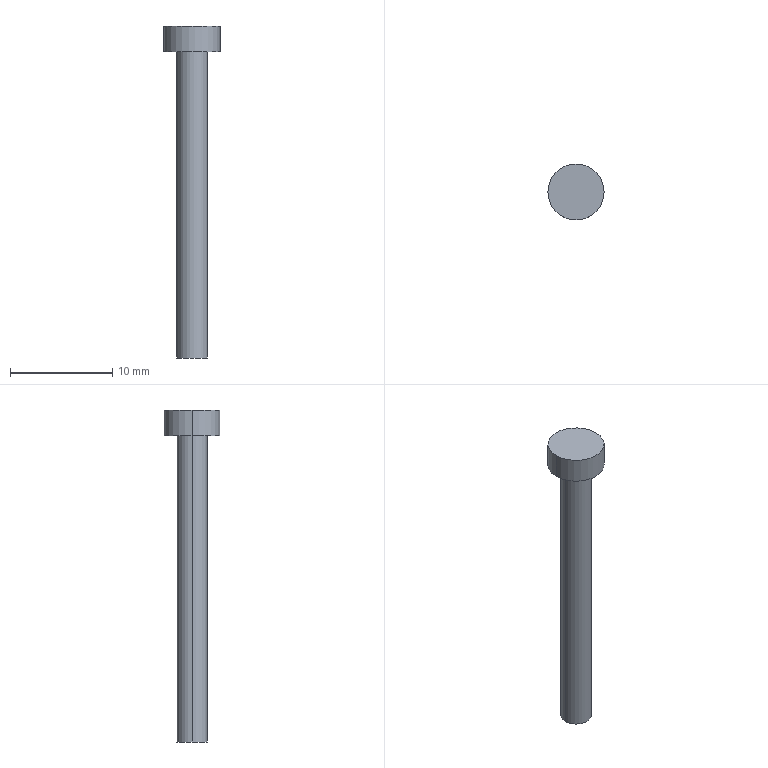Part | SolidWorks | features Extrusion 1, ICE 1 | 1 solid | 7 faces | box 5.5 x 5.5 x 32.5 mm | volume 271.453 mm3 | cylinder 4 | plane 3 | commonest cylinder face diameters 3 x2 5.5 x2
STEP:
#1=CARTESIAN_POINT('',(2.75,0.,2.5));
#2=VERTEX_POINT('',#1);
#3=CARTESIAN_POINT('',(-2.75,0.,2.5));
#4=VERTEX_POINT('',#3);
#5=CARTESIAN_POINT('',(0.,0.,2.5));
#6=DIRECTION('',(0.,0.,1.));
#7=DIRECTION('',(1.,0.,0.));
#8=AXIS2_PLACEMENT_3D('',#5,#6,#7);
#9=CIRCLE('',#8,2.75);
#10=EDGE_CURVE('',#2,#4,#9,.T.);
#11=ORIENTED_EDGE('',*,*,#10,.F.);
#12=CARTESIAN_POINT('',(2.75,0.,0.));
#13=VERTEX_POINT('',#12);
#14=CARTESIAN_POINT('',(2.75,0.,2.5));
#15=DIRECTION('',(0.,0.,-1.));
#16=VECTOR('',#15,1000.);
#17=LINE('',#14,#16);
#18=EDGE_CURVE('',#2,#13,#17,.T.);
#19=ORIENTED_EDGE('',*,*,#18,.T.);
#20=CARTESIAN_POINT('',(-2.75,0.,0.));
#21=VERTEX_POINT('',#20);
#22=CARTESIAN_POINT('',(0.,0.,0.));
#23=DIRECTION('',(0.,0.,1.));
#24=DIRECTION('',(1.,0.,0.));
#25=AXIS2_PLACEMENT_3D('',#22,#23,#24);
#26=CIRCLE('',#25,2.75);
#27=EDGE_CURVE('',#13,#21,#26,.T.);
#28=ORIENTED_EDGE('',*,*,#27,.T.);
#29=CARTESIAN_POINT('',(-2.75,0.,2.5));
#30=DIRECTION('',(0.,0.,-1.));
#31=VECTOR('',#30,1000.);
#32=LINE('',#29,#31);
#33=EDGE_CURVE('',#4,#21,#32,.T.);
#34=ORIENTED_EDGE('',*,*,#33,.F.);
#35=EDGE_LOOP('',(#11,#19,#28,#34));
#36=FACE_OUTER_BOUND('',#35,.T.);
#37=CARTESIAN_POINT('',(0.,0.,2.5));
#38=DIRECTION('',(0.,0.,-1.));
#39=DIRECTION('',(-1.,0.,0.));
#40=AXIS2_PLACEMENT_3D('',#37,#38,#39);
#41=CYLINDRICAL_SURFACE('',#40,2.75);
#42=ADVANCED_FACE('',(#36),#41,.T.);
#43=CARTESIAN_POINT('',(1.5,0.,-30.));
#44=VERTEX_POINT('',#43);
#45=CARTESIAN_POINT('',(-1.5,0.,-30.));
#46=VERTEX_POINT('',#45);
#47=CARTESIAN_POINT('',(0.,0.,-30.));
#48=DIRECTION('',(0.,0.,1.));
#49=DIRECTION('',(1.,0.,0.));
#50=AXIS2_PLACEMENT_3D('',#47,#48,#49);
#51=CIRCLE('',#50,1.5);
#52=EDGE_CURVE('',#44,#46,#51,.T.);
#53=ORIENTED_EDGE('',*,*,#52,.T.);
#54=CARTESIAN_POINT('',(-1.5,0.,0.));
#55=VERTEX_POINT('',#54);
#56=CARTESIAN_POINT('',(-1.5,0.,-30.));
#57=DIRECTION('',(0.,0.,1.));
#58=VECTOR('',#57,1000.);
#59=LINE('',#56,#58);
#60=EDGE_CURVE('',#46,#55,#59,.T.);
#61=ORIENTED_EDGE('',*,*,#60,.T.);
#62=CARTESIAN_POINT('',(1.5,0.,0.));
#63=VERTEX_POINT('',#62);
#64=CARTESIAN_POINT('',(0.,0.,0.));
#65=DIRECTION('',(0.,0.,1.));
#66=DIRECTION('',(1.,0.,0.));
#67=AXIS2_PLACEMENT_3D('',#64,#65,#66);
#68=CIRCLE('',#67,1.5);
#69=EDGE_CURVE('',#63,#55,#68,.T.);
#70=ORIENTED_EDGE('',*,*,#69,.F.);
#71=CARTESIAN_POINT('',(1.5,0.,-30.));
#72=DIRECTION('',(0.,0.,1.));
#73=VECTOR('',#72,1000.);
#74=LINE('',#71,#73);
#75=EDGE_CURVE('',#44,#63,#74,.T.);
#76=ORIENTED_EDGE('',*,*,#75,.F.);
#77=EDGE_LOOP('',(#53,#61,#70,#76));
#78=FACE_OUTER_BOUND('',#77,.T.);
#79=CARTESIAN_POINT('',(0.,0.,-30.));
#80=DIRECTION('',(0.,0.,1.));
#81=DIRECTION('',(1.,0.,0.));
#82=AXIS2_PLACEMENT_3D('',#79,#80,#81);
#83=CYLINDRICAL_SURFACE('',#82,1.5);
#84=ADVANCED_FACE('',(#78),#83,.T.);
#85=ORIENTED_EDGE('',*,*,#60,.F.);
#86=CARTESIAN_POINT('',(0.,0.,-30.));
#87=DIRECTION('',(0.,0.,1.));
#88=DIRECTION('',(1.,0.,0.));
#89=AXIS2_PLACEMENT_3D('',#86,#87,#88);
#90=CIRCLE('',#89,1.5);
#91=EDGE_CURVE('',#46,#44,#90,.T.);
#92=ORIENTED_EDGE('',*,*,#91,.T.);
#93=ORIENTED_EDGE('',*,*,#75,.T.);
#94=CARTESIAN_POINT('',(0.,0.,0.));
#95=DIRECTION('',(0.,0.,1.));
#96=DIRECTION('',(1.,0.,0.));
#97=AXIS2_PLACEMENT_3D('',#94,#95,#96);
#98=CIRCLE('',#97,1.5);
#99=EDGE_CURVE('',#55,#63,#98,.T.);
#100=ORIENTED_EDGE('',*,*,#99,.F.);
#101=EDGE_LOOP('',(#85,#92,#93,#100));
#102=FACE_OUTER_BOUND('',#101,.T.);
#103=CARTESIAN_POINT('',(0.,0.,-30.));
#104=DIRECTION('',(0.,0.,1.));
#105=DIRECTION('',(1.,0.,0.));
#106=AXIS2_PLACEMENT_3D('',#103,#104,#105);
#107=CYLINDRICAL_SURFACE('',#106,1.5);
#108=ADVANCED_FACE('',(#102),#107,.T.);
#109=ORIENTED_EDGE('',*,*,#52,.F.);
#110=ORIENTED_EDGE('',*,*,#91,.F.);
#111=EDGE_LOOP('',(#109,#110));
#112=FACE_OUTER_BOUND('',#111,.T.);
#113=CARTESIAN_POINT('',(0.,0.,-30.));
#114=DIRECTION('',(0.,0.,1.));
#115=DIRECTION('',(1.,0.,0.));
#116=AXIS2_PLACEMENT_3D('',#113,#114,#115);
#117=PLANE('',#116);
#118=ADVANCED_FACE('',(#112),#117,.F.);
#119=ORIENTED_EDGE('',*,*,#18,.F.);
#120=CARTESIAN_POINT('',(0.,0.,2.5));
#121=DIRECTION('',(0.,0.,1.));
#122=DIRECTION('',(1.,0.,0.));
#123=AXIS2_PLACEMENT_3D('',#120,#121,#122);
#124=CIRCLE('',#123,2.75);
#125=EDGE_CURVE('',#4,#2,#124,.T.);
#126=ORIENTED_EDGE('',*,*,#125,.F.);
#127=ORIENTED_EDGE('',*,*,#33,.T.);
#128=CARTESIAN_POINT('',(0.,0.,0.));
#129=DIRECTION('',(0.,0.,1.));
#130=DIRECTION('',(1.,0.,0.));
#131=AXIS2_PLACEMENT_3D('',#128,#129,#130);
#132=CIRCLE('',#131,2.75);
#133=EDGE_CURVE('',#21,#13,#132,.T.);
#134=ORIENTED_EDGE('',*,*,#133,.T.);
#135=EDGE_LOOP('',(#119,#126,#127,#134));
#136=FACE_OUTER_BOUND('',#135,.T.);
#137=CARTESIAN_POINT('',(0.,0.,2.5));
#138=DIRECTION('',(0.,0.,-1.));
#139=DIRECTION('',(-1.,0.,0.));
#140=AXIS2_PLACEMENT_3D('',#137,#138,#139);
#141=CYLINDRICAL_SURFACE('',#140,2.75);
#142=ADVANCED_FACE('',(#136),#141,.T.);
#143=ORIENTED_EDGE('',*,*,#125,.T.);
#144=ORIENTED_EDGE('',*,*,#10,.T.);
#145=EDGE_LOOP('',(#143,#144));
#146=FACE_OUTER_BOUND('',#145,.T.);
#147=CARTESIAN_POINT('',(0.,0.,2.5));
#148=DIRECTION('',(0.,0.,1.));
#149=DIRECTION('',(1.,0.,0.));
#150=AXIS2_PLACEMENT_3D('',#147,#148,#149);
#151=PLANE('',#150);
#152=ADVANCED_FACE('',(#146),#151,.T.);
#153=ORIENTED_EDGE('',*,*,#69,.T.);
#154=ORIENTED_EDGE('',*,*,#99,.T.);
#155=EDGE_LOOP('',(#153,#154));
#156=FACE_BOUND('',#155,.T.);
#157=ORIENTED_EDGE('',*,*,#133,.F.);
#158=ORIENTED_EDGE('',*,*,#27,.F.);
#159=EDGE_LOOP('',(#157,#158));
#160=FACE_OUTER_BOUND('',#159,.T.);
#161=CARTESIAN_POINT('',(0.,0.,0.));
#162=DIRECTION('',(0.,0.,1.));
#163=DIRECTION('',(1.,0.,0.));
#164=AXIS2_PLACEMENT_3D('',#161,#162,#163);
#165=PLANE('',#164);
#166=ADVANCED_FACE('',(#156,#160),#165,.F.);
#167=CLOSED_SHELL('',(#42,#84,#108,#118,#142,#152,#166));
#168=MANIFOLD_SOLID_BREP('',#167);
#169=CARTESIAN_POINT('',(0.,0.,0.));
#170=DIRECTION('',(0.,0.,1.));
#171=DIRECTION('',(1.,0.,0.));
#172=AXIS2_PLACEMENT_3D('',#169,#170,#171);
#173=(LENGTH_UNIT()NAMED_UNIT(*)SI_UNIT(.MILLI.,.METRE.));
#174=UNCERTAINTY_MEASURE_WITH_UNIT(LENGTH_MEASURE(0.00001),#173,'','');
#175=(NAMED_UNIT(*)PLANE_ANGLE_UNIT()SI_UNIT($,.RADIAN.));
#176=(NAMED_UNIT(*)SI_UNIT($,.STERADIAN.)SOLID_ANGLE_UNIT());
#177=(GEOMETRIC_REPRESENTATION_CONTEXT(3)GLOBAL_UNCERTAINTY_ASSIGNED_CONTEXT((#174))GLOBAL_UNIT_ASSIGNED_CONTEXT((#173,#175,#176))REPRESENTATION_CONTEXT('',''));
#178=ADVANCED_BREP_SHAPE_REPRESENTATION('',(#168,#172),#177);